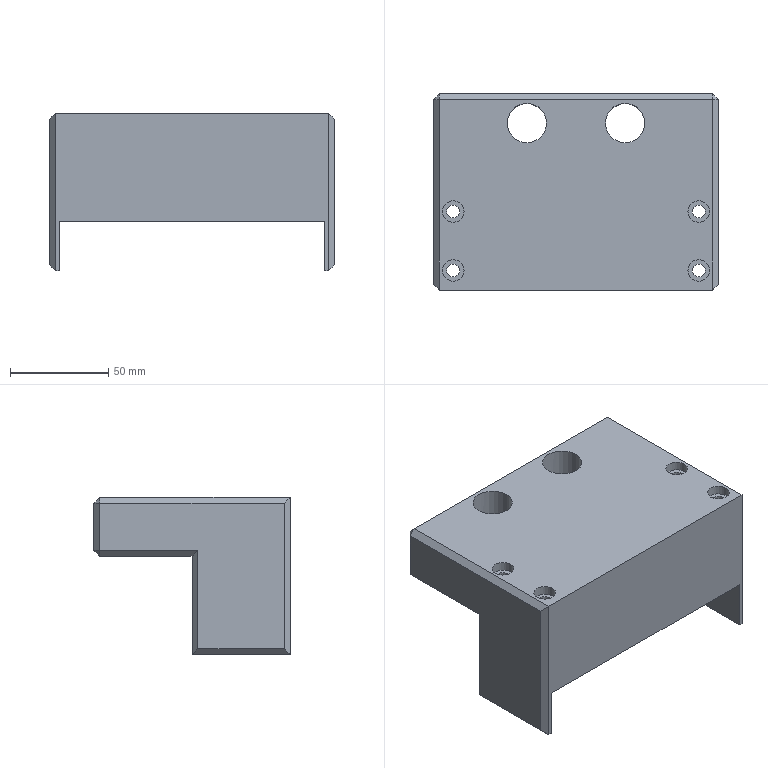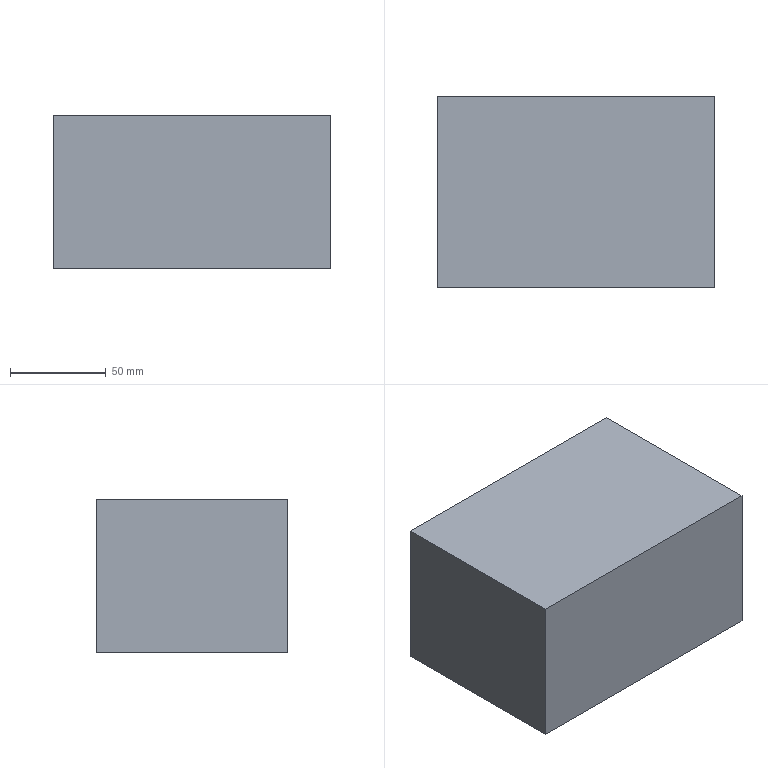CAM job | NX | 3+2 milling, drilling | part box 145 x 100 x 80 mm | stock box 145 x 100 x 80 mm
Tools:
number,name,description,diameter,corner_radius,flute_length,length,flutes
6,D8A45,Milling Tool-5 Parameters,8.0,0.0,4.0,4.0,2
15,6.6ZT,Drilling Tool,6.6,0.0,35.0,50.0,2
17,10.5ZT,Drilling Tool,10.5,0.0,35.0,50.0,2
4,D10JING,Milling Tool-5 Parameters,10.0,0.0,50.0,75.0,2
2,D6,Milling Tool-5 Parameters,6.0,0.0,50.0,75.0,2
1,D63,Milling Tool-5 Parameters,63.0,0.0,50.0,75.0,2
14,5.0ZT,Drilling Tool,5.0,0.0,35.0,50.0,2
Operations:
program,operation,operation_type,tool,method,geometry_group,spindle_rpm,surface_speed,feed_per_tooth,feed_cut,feed_plunge,cut_length_mm,path_length_mm,cut_time_min,machine_time_min
1,DRILLING_COPY_2,Operation,D8A45,METHOD,A,3000.0,56.0,0.025,150.0,0.0,24.0,350.697,0.16,0.1927
1,DRILLING_COPY_COPY_COPY_COPY_1_COPY,Operation,6.6ZT,METHOD,A,2000.0,20.0,0.0375,150.0,0.0,245.931,746.198,1.639,1.69
1,DRILLING_COPY_COPY_COPY_COPY_1_COPY_COPY,Operation,10.5ZT,METHOD,A,1000.0,32.0,0.075,150.0,0.0,75.309,263.708,0.5021,0.5209
1,刀补12_COPY,CylinderMilling,D10JING,METHOD,A,7000.0,219.0,0.0857,1200.0,100.0,1971.397,2200.397,1.643,1.666
1,HOLE_MILLING,CylinderMilling,D6,METHOD,A,8000.0,301.0,0.0625,1000.0,100.0,748.03,1193.38,0.748,0.7926
1,ZLEVEL_PROFILE_1_COPY_1_COPY_COPY_1_COPY_COPY,ZLevelMilling,D8A45,METHOD,A,7500.0,141.0,0.0667,1000.0,100.0,272.09,1165.168,0.2721,0.3614
1,ZLEVEL_PROFILE_1_COPY_1_COPY_COPY_1_COPY_COPY_COPY,ZLevelMilling,D8A45,METHOD,A,7500.0,141.0,0.0667,1000.0,100.0,500.236,565.236,0.5002,0.5067
1,刀补12,CylinderMilling,D10JING,METHOD,A,8000.0,301.0,0.0625,1000.0,100.0,575.189,804.189,0.5752,0.5981
2,FLOOR_WALL_2,VolumeBased25DMillingOperation,D63,METHOD,B,6500.0,1286.0,0.1154,1500.0,1000.0,11224.434,27360.425,7.618,9.232
2,FLOOR_WALL_1_COPY_COPY_COPY_COPY,VolumeBased25DMillingOperation,D10JING,METHOD,B,7500.0,235.0,0.0833,1250.0,100.0,830.556,2046.956,0.6644,0.7861
2,FLOOR_WALL_1_COPY_COPY_COPY,VolumeBased25DMillingOperation,D10JING,METHOD,B,7500.0,235.0,0.0833,1250.0,100.0,1765.495,2243.9,1.412,1.46
2,DRILLING_COPY_2_COPY,Operation,D8A45,METHOD,B,3000.0,56.0,0.025,150.0,0.0,12.0,137.09,0.08,0.0925
2,DRILLING_COPY_COPY_COPY_COPY_1_COPY_COPY_1,Operation,5.0ZT,METHOD,B,2000.0,20.0,0.0375,150.0,0.0,22.639,158.369,0.1509,0.1645
2,ZLEVEL_PROFILE_1_COPY_1_COPY_COPY_1_COPY_COPY_COPY_COPY,ZLevelMilling,D8A45,METHOD,B,7500.0,141.0,0.0667,1000.0,100.0,354.24,419.24,0.3542,0.3607
2,ZLEVEL_PROFILE_1_COPY_1_COPY_COPY_1_COPY_COPY_COPY_COPY_COPY,ZLevelMilling,D8A45,METHOD,B,7500.0,141.0,0.0667,1000.0,100.0,298.567,463.567,0.2986,0.3151
2,ZLEVEL_PROFILE_1_COPY_1_COPY_COPY_1_COPY_COPY_COPY_COPY_COPY_COPY,ZLevelMilling,D8A45,METHOD,B,7500.0,141.0,0.0667,1000.0,100.0,483.543,658.625,0.4835,0.5011
3,FLOOR_WALL_2_COPY,VolumeBased25DMillingOperation,D63,METHOD,C,6500.0,1286.0,0.1154,1500.0,1000.0,10672.292,16180.518,7.182,7.733
3,FLOOR_WALL_1_COPY_COPY_COPY_COPY_COPY,VolumeBased25DMillingOperation,D10JING,METHOD,C,7500.0,235.0,0.0833,1250.0,100.0,269.615,953.902,0.2157,0.2841
3,FLOOR_WALL_1_COPY_COPY_COPY_COPY_1,VolumeBased25DMillingOperation,D10JING,METHOD,C,7500.0,235.0,0.0833,1250.0,100.0,1827.988,2271.292,1.462,1.507
3,ZLEVEL_PROFILE_1_COPY_1_COPY_COPY_1_COPY_COPY_COPY_COPY_COPY_1,ZLevelMilling,D8A45,METHOD,C,7500.0,141.0,0.0667,1000.0,100.0,277.002,566.201,0.277,0.3059
3,ZLEVEL_PROFILE_1_COPY_1_COPY_COPY_1_COPY_COPY_COPY_COPY_COPY_1_COPY,ZLevelMilling,D8A45,METHOD,C,7500.0,141.0,0.0667,1000.0,100.0,264.353,551.626,0.2644,0.2931
3,ZLEVEL_PROFILE_1_COPY_1_COPY_COPY_1_COPY_COPY_COPY_COPY_COPY_1_COPY_COPY,ZLevelMilling,D8A45,METHOD,C,7500.0,141.0,0.0667,1000.0,100.0,327.954,1272.606,0.328,0.4224
3,ZLEVEL_PROFILE_1_COPY_1_COPY_COPY_1_COPY_COPY_COPY_COPY_COPY_1_COPY_COPY_COPY,ZLevelMilling,D8A45,METHOD,C,7500.0,141.0,0.0667,1000.0,100.0,127.705,500.645,0.1277,0.165